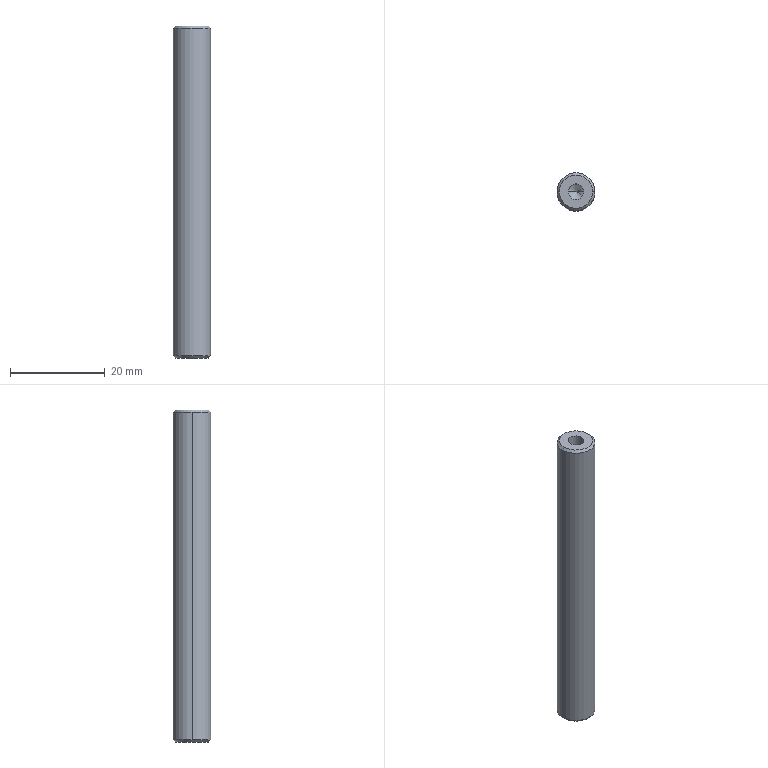Part | STEP file | 01-06 sliding guide post | 1 solid | 12 faces | box 8 x 8 x 70 mm | volume 3411 mm3 | cone 6 | cylinder 4 | plane 2 | commonest cylinder face diameters 3.3 x2 8 x2
STEP:
#1=CARTESIAN_POINT('',(-1.65,0.,58.5));
#2=VERTEX_POINT('',#1);
#3=CARTESIAN_POINT('',(1.65,0.,58.5));
#4=VERTEX_POINT('',#3);
#5=CARTESIAN_POINT('',(0.,0.,58.5));
#6=DIRECTION('',(0.,0.,1.));
#7=DIRECTION('',(1.,0.,0.));
#8=AXIS2_PLACEMENT_3D('',#5,#6,#7);
#9=CIRCLE('',#8,1.65);
#10=EDGE_CURVE('',#2,#4,#9,.T.);
#11=ORIENTED_EDGE('',*,*,#10,.F.);
#12=CARTESIAN_POINT('',(-1.65,0.,70.));
#13=VERTEX_POINT('',#12);
#14=CARTESIAN_POINT('',(-1.65,0.,70.));
#15=DIRECTION('',(0.,0.,1.));
#16=VECTOR('',#15,1000.);
#17=LINE('',#14,#16);
#18=EDGE_CURVE('',#2,#13,#17,.T.);
#19=ORIENTED_EDGE('',*,*,#18,.T.);
#20=CARTESIAN_POINT('',(1.65,0.,70.));
#21=VERTEX_POINT('',#20);
#22=CARTESIAN_POINT('',(0.,0.,70.));
#23=DIRECTION('',(0.,0.,1.));
#24=DIRECTION('',(1.,0.,0.));
#25=AXIS2_PLACEMENT_3D('',#22,#23,#24);
#26=CIRCLE('',#25,1.65);
#27=EDGE_CURVE('',#13,#21,#26,.T.);
#28=ORIENTED_EDGE('',*,*,#27,.T.);
#29=CARTESIAN_POINT('',(1.65,0.,70.));
#30=DIRECTION('',(0.,0.,1.));
#31=VECTOR('',#30,1000.);
#32=LINE('',#29,#31);
#33=EDGE_CURVE('',#4,#21,#32,.T.);
#34=ORIENTED_EDGE('',*,*,#33,.F.);
#35=EDGE_LOOP('',(#11,#19,#28,#34));
#36=FACE_OUTER_BOUND('',#35,.T.);
#37=CARTESIAN_POINT('',(0.,0.,70.));
#38=DIRECTION('',(0.,0.,1.));
#39=DIRECTION('',(1.,0.,0.));
#40=AXIS2_PLACEMENT_3D('',#37,#38,#39);
#41=CYLINDRICAL_SURFACE('',#40,1.65);
#42=ADVANCED_FACE('',(#36),#41,.F.);
#43=CARTESIAN_POINT('',(0.,0.,57.509));
#44=VERTEX_POINT('',#43);
#45=CARTESIAN_POINT('',(1.65,0.,58.5));
#46=DIRECTION('',(0.8572,0.,0.515));
#47=VECTOR('',#46,1000.);
#48=LINE('',#45,#47);
#49=EDGE_CURVE('',#44,#4,#48,.T.);
#50=ORIENTED_EDGE('',*,*,#49,.F.);
#51=CARTESIAN_POINT('',(-1.65,0.,58.5));
#52=DIRECTION('',(-0.8572,0.,0.515));
#53=VECTOR('',#52,1000.);
#54=LINE('',#51,#53);
#55=EDGE_CURVE('',#44,#2,#54,.T.);
#56=ORIENTED_EDGE('',*,*,#55,.T.);
#57=ORIENTED_EDGE('',*,*,#10,.T.);
#58=EDGE_LOOP('',(#50,#56,#57));
#59=FACE_OUTER_BOUND('',#58,.T.);
#60=CARTESIAN_POINT('',(0.,0.,58.5));
#61=DIRECTION('',(0.,0.,1.));
#62=DIRECTION('',(1.,0.,0.));
#63=AXIS2_PLACEMENT_3D('',#60,#61,#62);
#64=CONICAL_SURFACE('',#63,1.65,1.03);
#65=ADVANCED_FACE('',(#59),#64,.F.);
#66=CARTESIAN_POINT('',(-3.5,0.,0.));
#67=VERTEX_POINT('',#66);
#68=CARTESIAN_POINT('',(3.5,0.,0.));
#69=VERTEX_POINT('',#68);
#70=CARTESIAN_POINT('',(0.,0.,0.));
#71=DIRECTION('',(0.,0.,-1.));
#72=DIRECTION('',(1.,0.,0.));
#73=AXIS2_PLACEMENT_3D('',#70,#71,#72);
#74=CIRCLE('',#73,3.5);
#75=EDGE_CURVE('',#67,#69,#74,.T.);
#76=ORIENTED_EDGE('',*,*,#75,.F.);
#77=CARTESIAN_POINT('',(-4.,0.,0.5));
#78=VERTEX_POINT('',#77);
#79=CARTESIAN_POINT('',(-4.,0.,0.5));
#80=DIRECTION('',(-0.7071,0.,0.7071));
#81=VECTOR('',#80,1000.);
#82=LINE('',#79,#81);
#83=EDGE_CURVE('',#67,#78,#82,.T.);
#84=ORIENTED_EDGE('',*,*,#83,.T.);
#85=CARTESIAN_POINT('',(4.,0.,0.5));
#86=VERTEX_POINT('',#85);
#87=CARTESIAN_POINT('',(0.,0.,0.5));
#88=DIRECTION('',(0.,0.,1.));
#89=DIRECTION('',(1.,0.,0.));
#90=AXIS2_PLACEMENT_3D('',#87,#88,#89);
#91=CIRCLE('',#90,4.);
#92=EDGE_CURVE('',#86,#78,#91,.T.);
#93=ORIENTED_EDGE('',*,*,#92,.F.);
#94=CARTESIAN_POINT('',(4.,0.,0.5));
#95=DIRECTION('',(0.7071,0.,0.7071));
#96=VECTOR('',#95,1000.);
#97=LINE('',#94,#96);
#98=EDGE_CURVE('',#69,#86,#97,.T.);
#99=ORIENTED_EDGE('',*,*,#98,.F.);
#100=EDGE_LOOP('',(#76,#84,#93,#99));
#101=FACE_OUTER_BOUND('',#100,.T.);
#102=CARTESIAN_POINT('',(0.,0.,0.5));
#103=DIRECTION('',(0.,0.,1.));
#104=DIRECTION('',(1.,0.,0.));
#105=AXIS2_PLACEMENT_3D('',#102,#103,#104);
#106=CONICAL_SURFACE('',#105,4.,0.7854);
#107=ADVANCED_FACE('',(#101),#106,.T.);
#108=CARTESIAN_POINT('',(3.5,0.,70.));
#109=VERTEX_POINT('',#108);
#110=CARTESIAN_POINT('',(-3.5,0.,70.));
#111=VERTEX_POINT('',#110);
#112=CARTESIAN_POINT('',(0.,0.,70.));
#113=DIRECTION('',(0.,0.,1.));
#114=DIRECTION('',(1.,0.,0.));
#115=AXIS2_PLACEMENT_3D('',#112,#113,#114);
#116=CIRCLE('',#115,3.5);
#117=EDGE_CURVE('',#109,#111,#116,.T.);
#118=ORIENTED_EDGE('',*,*,#117,.F.);
#119=CARTESIAN_POINT('',(4.,0.,69.5));
#120=VERTEX_POINT('',#119);
#121=CARTESIAN_POINT('',(3.5,0.,70.));
#122=DIRECTION('',(0.7071,0.,-0.7071));
#123=VECTOR('',#122,1000.);
#124=LINE('',#121,#123);
#125=EDGE_CURVE('',#109,#120,#124,.T.);
#126=ORIENTED_EDGE('',*,*,#125,.T.);
#127=CARTESIAN_POINT('',(-4.,0.,69.5));
#128=VERTEX_POINT('',#127);
#129=CARTESIAN_POINT('',(0.,0.,69.5));
#130=DIRECTION('',(0.,0.,-1.));
#131=DIRECTION('',(1.,0.,0.));
#132=AXIS2_PLACEMENT_3D('',#129,#130,#131);
#133=CIRCLE('',#132,4.);
#134=EDGE_CURVE('',#128,#120,#133,.T.);
#135=ORIENTED_EDGE('',*,*,#134,.F.);
#136=CARTESIAN_POINT('',(-3.5,0.,70.));
#137=DIRECTION('',(-0.7071,0.,-0.7071));
#138=VECTOR('',#137,1000.);
#139=LINE('',#136,#138);
#140=EDGE_CURVE('',#111,#128,#139,.T.);
#141=ORIENTED_EDGE('',*,*,#140,.F.);
#142=EDGE_LOOP('',(#118,#126,#135,#141));
#143=FACE_OUTER_BOUND('',#142,.T.);
#144=CARTESIAN_POINT('',(0.,0.,70.));
#145=DIRECTION('',(0.,0.,-1.));
#146=DIRECTION('',(-1.,0.,0.));
#147=AXIS2_PLACEMENT_3D('',#144,#145,#146);
#148=CONICAL_SURFACE('',#147,3.5,0.7854);
#149=ADVANCED_FACE('',(#143),#148,.T.);
#150=ORIENTED_EDGE('',*,*,#134,.T.);
#151=CARTESIAN_POINT('',(4.,0.,70.));
#152=DIRECTION('',(0.,0.,-1.));
#153=VECTOR('',#152,1000.);
#154=LINE('',#151,#153);
#155=EDGE_CURVE('',#120,#86,#154,.T.);
#156=ORIENTED_EDGE('',*,*,#155,.T.);
#157=ORIENTED_EDGE('',*,*,#92,.T.);
#158=CARTESIAN_POINT('',(-4.,0.,70.));
#159=DIRECTION('',(0.,0.,-1.));
#160=VECTOR('',#159,1000.);
#161=LINE('',#158,#160);
#162=EDGE_CURVE('',#128,#78,#161,.T.);
#163=ORIENTED_EDGE('',*,*,#162,.F.);
#164=EDGE_LOOP('',(#150,#156,#157,#163));
#165=FACE_OUTER_BOUND('',#164,.T.);
#166=CARTESIAN_POINT('',(0.,0.,70.));
#167=DIRECTION('',(0.,0.,-1.));
#168=DIRECTION('',(-1.,0.,0.));
#169=AXIS2_PLACEMENT_3D('',#166,#167,#168);
#170=CYLINDRICAL_SURFACE('',#169,4.);
#171=ADVANCED_FACE('',(#165),#170,.T.);
#172=ORIENTED_EDGE('',*,*,#155,.F.);
#173=CARTESIAN_POINT('',(0.,0.,69.5));
#174=DIRECTION('',(0.,0.,-1.));
#175=DIRECTION('',(1.,0.,0.));
#176=AXIS2_PLACEMENT_3D('',#173,#174,#175);
#177=CIRCLE('',#176,4.);
#178=EDGE_CURVE('',#120,#128,#177,.T.);
#179=ORIENTED_EDGE('',*,*,#178,.T.);
#180=ORIENTED_EDGE('',*,*,#162,.T.);
#181=CARTESIAN_POINT('',(0.,0.,0.5));
#182=DIRECTION('',(0.,0.,1.));
#183=DIRECTION('',(1.,0.,0.));
#184=AXIS2_PLACEMENT_3D('',#181,#182,#183);
#185=CIRCLE('',#184,4.);
#186=EDGE_CURVE('',#78,#86,#185,.T.);
#187=ORIENTED_EDGE('',*,*,#186,.T.);
#188=EDGE_LOOP('',(#172,#179,#180,#187));
#189=FACE_OUTER_BOUND('',#188,.T.);
#190=CARTESIAN_POINT('',(0.,0.,70.));
#191=DIRECTION('',(0.,0.,-1.));
#192=DIRECTION('',(-1.,0.,0.));
#193=AXIS2_PLACEMENT_3D('',#190,#191,#192);
#194=CYLINDRICAL_SURFACE('',#193,4.);
#195=ADVANCED_FACE('',(#189),#194,.T.);
#196=CARTESIAN_POINT('',(0.,0.,70.));
#197=DIRECTION('',(0.,0.,1.));
#198=DIRECTION('',(1.,0.,0.));
#199=AXIS2_PLACEMENT_3D('',#196,#197,#198);
#200=CIRCLE('',#199,1.65);
#201=EDGE_CURVE('',#21,#13,#200,.T.);
#202=ORIENTED_EDGE('',*,*,#201,.F.);
#203=ORIENTED_EDGE('',*,*,#27,.F.);
#204=EDGE_LOOP('',(#202,#203));
#205=FACE_BOUND('',#204,.T.);
#206=CARTESIAN_POINT('',(0.,0.,70.));
#207=DIRECTION('',(0.,0.,1.));
#208=DIRECTION('',(1.,0.,0.));
#209=AXIS2_PLACEMENT_3D('',#206,#207,#208);
#210=CIRCLE('',#209,3.5);
#211=EDGE_CURVE('',#111,#109,#210,.T.);
#212=ORIENTED_EDGE('',*,*,#211,.T.);
#213=ORIENTED_EDGE('',*,*,#117,.T.);
#214=EDGE_LOOP('',(#212,#213));
#215=FACE_OUTER_BOUND('',#214,.T.);
#216=CARTESIAN_POINT('',(0.,0.,70.));
#217=DIRECTION('',(0.,0.,1.));
#218=DIRECTION('',(1.,0.,0.));
#219=AXIS2_PLACEMENT_3D('',#216,#217,#218);
#220=PLANE('',#219);
#221=ADVANCED_FACE('',(#205,#215),#220,.T.);
#222=CARTESIAN_POINT('',(0.,0.,0.));
#223=DIRECTION('',(0.,0.,-1.));
#224=DIRECTION('',(1.,0.,0.));
#225=AXIS2_PLACEMENT_3D('',#222,#223,#224);
#226=CIRCLE('',#225,3.5);
#227=EDGE_CURVE('',#69,#67,#226,.T.);
#228=ORIENTED_EDGE('',*,*,#227,.T.);
#229=ORIENTED_EDGE('',*,*,#75,.T.);
#230=EDGE_LOOP('',(#228,#229));
#231=FACE_OUTER_BOUND('',#230,.T.);
#232=CARTESIAN_POINT('',(0.,0.,0.));
#233=DIRECTION('',(0.,0.,1.));
#234=DIRECTION('',(1.,0.,0.));
#235=AXIS2_PLACEMENT_3D('',#232,#233,#234);
#236=PLANE('',#235);
#237=ADVANCED_FACE('',(#231),#236,.F.);
#238=ORIENTED_EDGE('',*,*,#125,.F.);
#239=ORIENTED_EDGE('',*,*,#211,.F.);
#240=ORIENTED_EDGE('',*,*,#140,.T.);
#241=ORIENTED_EDGE('',*,*,#178,.F.);
#242=EDGE_LOOP('',(#238,#239,#240,#241));
#243=FACE_OUTER_BOUND('',#242,.T.);
#244=CARTESIAN_POINT('',(0.,0.,70.));
#245=DIRECTION('',(0.,0.,-1.));
#246=DIRECTION('',(-1.,0.,0.));
#247=AXIS2_PLACEMENT_3D('',#244,#245,#246);
#248=CONICAL_SURFACE('',#247,3.5,0.7854);
#249=ADVANCED_FACE('',(#243),#248,.T.);
#250=ORIENTED_EDGE('',*,*,#83,.F.);
#251=ORIENTED_EDGE('',*,*,#227,.F.);
#252=ORIENTED_EDGE('',*,*,#98,.T.);
#253=ORIENTED_EDGE('',*,*,#186,.F.);
#254=EDGE_LOOP('',(#250,#251,#252,#253));
#255=FACE_OUTER_BOUND('',#254,.T.);
#256=CARTESIAN_POINT('',(0.,0.,0.5));
#257=DIRECTION('',(0.,0.,1.));
#258=DIRECTION('',(1.,0.,0.));
#259=AXIS2_PLACEMENT_3D('',#256,#257,#258);
#260=CONICAL_SURFACE('',#259,4.,0.7854);
#261=ADVANCED_FACE('',(#255),#260,.T.);
#262=ORIENTED_EDGE('',*,*,#55,.F.);
#263=ORIENTED_EDGE('',*,*,#49,.T.);
#264=CARTESIAN_POINT('',(0.,0.,58.5));
#265=DIRECTION('',(0.,0.,1.));
#266=DIRECTION('',(1.,0.,0.));
#267=AXIS2_PLACEMENT_3D('',#264,#265,#266);
#268=CIRCLE('',#267,1.65);
#269=EDGE_CURVE('',#4,#2,#268,.T.);
#270=ORIENTED_EDGE('',*,*,#269,.T.);
#271=EDGE_LOOP('',(#262,#263,#270));
#272=FACE_OUTER_BOUND('',#271,.T.);
#273=CARTESIAN_POINT('',(0.,0.,58.5));
#274=DIRECTION('',(0.,0.,1.));
#275=DIRECTION('',(1.,0.,0.));
#276=AXIS2_PLACEMENT_3D('',#273,#274,#275);
#277=CONICAL_SURFACE('',#276,1.65,1.03);
#278=ADVANCED_FACE('',(#272),#277,.F.);
#279=ORIENTED_EDGE('',*,*,#18,.F.);
#280=ORIENTED_EDGE('',*,*,#269,.F.);
#281=ORIENTED_EDGE('',*,*,#33,.T.);
#282=ORIENTED_EDGE('',*,*,#201,.T.);
#283=EDGE_LOOP('',(#279,#280,#281,#282));
#284=FACE_OUTER_BOUND('',#283,.T.);
#285=CARTESIAN_POINT('',(0.,0.,70.));
#286=DIRECTION('',(0.,0.,1.));
#287=DIRECTION('',(1.,0.,0.));
#288=AXIS2_PLACEMENT_3D('',#285,#286,#287);
#289=CYLINDRICAL_SURFACE('',#288,1.65);
#290=ADVANCED_FACE('',(#284),#289,.F.);
#291=CLOSED_SHELL('',(#42,#65,#107,#149,#171,#195,#221,#237,#249,#261,#278,#290));
#292=MANIFOLD_SOLID_BREP('',#291);
#293=CARTESIAN_POINT('',(0.,0.,0.));
#294=DIRECTION('',(0.,0.,1.));
#295=DIRECTION('',(1.,0.,0.));
#296=AXIS2_PLACEMENT_3D('',#293,#294,#295);
#297=(LENGTH_UNIT()NAMED_UNIT(*)SI_UNIT(.MILLI.,.METRE.));
#298=UNCERTAINTY_MEASURE_WITH_UNIT(LENGTH_MEASURE(0.00001),#297,'','');
#299=(NAMED_UNIT(*)PLANE_ANGLE_UNIT()SI_UNIT($,.RADIAN.));
#300=(NAMED_UNIT(*)SI_UNIT($,.STERADIAN.)SOLID_ANGLE_UNIT());
#301=(GEOMETRIC_REPRESENTATION_CONTEXT(3)GLOBAL_UNCERTAINTY_ASSIGNED_CONTEXT((#298))GLOBAL_UNIT_ASSIGNED_CONTEXT((#297,#299,#300))REPRESENTATION_CONTEXT('',''));
#302=ADVANCED_BREP_SHAPE_REPRESENTATION('',(#292,#296),#301);